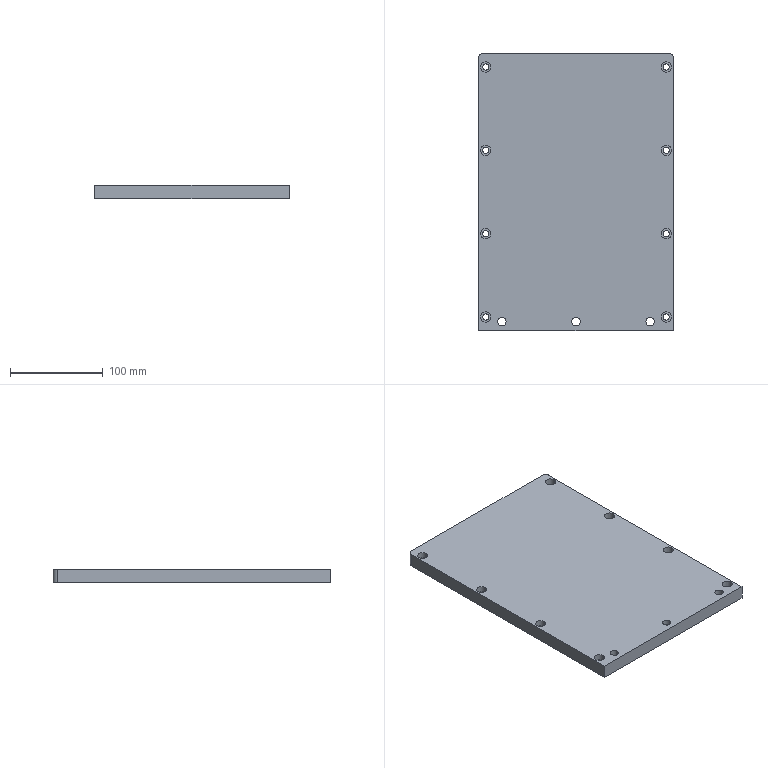Part | STEP file | KF-2212-050-001 | 1 solid | 63 faces | box 210 x 300 x 15 mm | volume 931509 mm3 | cylinder 46 | plane 17 | commonest cylinder face diameters 6.6 x16 11 x16 9 x6 15 x6 10 x2